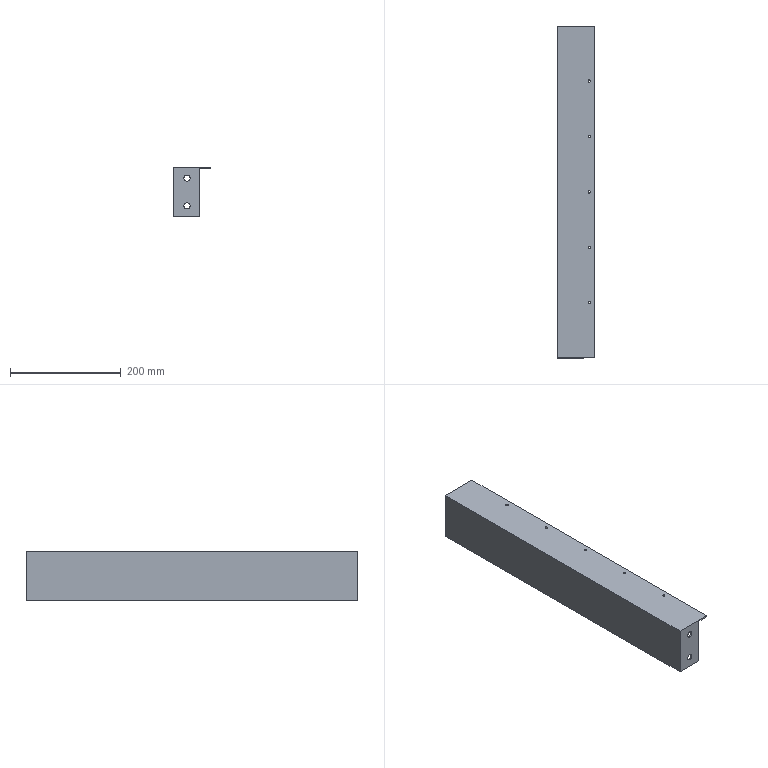Part | SolidWorks | features BaseBody 1 | 1 solid | 32 faces | box 68 x 599 x 90 mm | volume 277615 mm3 | cylinder 18 | plane 14 | commonest cylinder face diameters 4.4 x10 11 x8
STEP:
#1=CARTESIAN_POINT('',(202.746,-3340.973,1407.471));
#2=VERTEX_POINT('',#1);
#3=CARTESIAN_POINT('',(207.146,-3340.973,1407.471));
#4=VERTEX_POINT('',#3);
#5=CARTESIAN_POINT('',(204.946,-3340.973,1407.471));
#6=DIRECTION('',(0.,0.,1.));
#7=DIRECTION('',(1.,0.,0.));
#8=AXIS2_PLACEMENT_3D('',#5,#6,#7);
#9=CIRCLE('',#8,2.2);
#10=EDGE_CURVE('',#2,#4,#9,.T.);
#11=ORIENTED_EDGE('',*,*,#10,.F.);
#12=CARTESIAN_POINT('',(202.746,-3340.973,1409.971));
#13=VERTEX_POINT('',#12);
#14=CARTESIAN_POINT('',(202.746,-3340.973,1429.62));
#15=DIRECTION('',(0.,0.,1.));
#16=VECTOR('',#15,1000.);
#17=LINE('',#14,#16);
#18=EDGE_CURVE('',#2,#13,#17,.T.);
#19=ORIENTED_EDGE('',*,*,#18,.T.);
#20=CARTESIAN_POINT('',(207.146,-3340.973,1409.971));
#21=VERTEX_POINT('',#20);
#22=CARTESIAN_POINT('',(204.946,-3340.973,1409.971));
#23=DIRECTION('',(0.,0.,-1.));
#24=DIRECTION('',(1.,0.,0.));
#25=AXIS2_PLACEMENT_3D('',#22,#23,#24);
#26=CIRCLE('',#25,2.2);
#27=EDGE_CURVE('',#21,#13,#26,.T.);
#28=ORIENTED_EDGE('',*,*,#27,.F.);
#29=CARTESIAN_POINT('',(207.146,-3340.973,1429.62));
#30=DIRECTION('',(0.,0.,1.));
#31=VECTOR('',#30,1000.);
#32=LINE('',#29,#31);
#33=EDGE_CURVE('',#4,#21,#32,.T.);
#34=ORIENTED_EDGE('',*,*,#33,.F.);
#35=EDGE_LOOP('',(#11,#19,#28,#34));
#36=FACE_OUTER_BOUND('',#35,.T.);
#37=CARTESIAN_POINT('',(204.946,-3340.973,1429.62));
#38=DIRECTION('',(0.,0.,1.));
#39=DIRECTION('',(1.,0.,0.));
#40=AXIS2_PLACEMENT_3D('',#37,#38,#39);
#41=CYLINDRICAL_SURFACE('',#40,2.2);
#42=ADVANCED_FACE('',(#36),#41,.F.);
#43=CARTESIAN_POINT('',(202.746,-3140.973,1407.471));
#44=VERTEX_POINT('',#43);
#45=CARTESIAN_POINT('',(207.146,-3140.973,1407.471));
#46=VERTEX_POINT('',#45);
#47=CARTESIAN_POINT('',(204.946,-3140.973,1407.471));
#48=DIRECTION('',(0.,0.,1.));
#49=DIRECTION('',(1.,0.,0.));
#50=AXIS2_PLACEMENT_3D('',#47,#48,#49);
#51=CIRCLE('',#50,2.2);
#52=EDGE_CURVE('',#44,#46,#51,.T.);
#53=ORIENTED_EDGE('',*,*,#52,.F.);
#54=CARTESIAN_POINT('',(202.746,-3140.973,1409.971));
#55=VERTEX_POINT('',#54);
#56=CARTESIAN_POINT('',(202.746,-3140.973,1429.62));
#57=DIRECTION('',(0.,0.,1.));
#58=VECTOR('',#57,1000.);
#59=LINE('',#56,#58);
#60=EDGE_CURVE('',#44,#55,#59,.T.);
#61=ORIENTED_EDGE('',*,*,#60,.T.);
#62=CARTESIAN_POINT('',(207.146,-3140.973,1409.971));
#63=VERTEX_POINT('',#62);
#64=CARTESIAN_POINT('',(204.946,-3140.973,1409.971));
#65=DIRECTION('',(0.,0.,-1.));
#66=DIRECTION('',(1.,0.,0.));
#67=AXIS2_PLACEMENT_3D('',#64,#65,#66);
#68=CIRCLE('',#67,2.2);
#69=EDGE_CURVE('',#63,#55,#68,.T.);
#70=ORIENTED_EDGE('',*,*,#69,.F.);
#71=CARTESIAN_POINT('',(207.146,-3140.973,1429.62));
#72=DIRECTION('',(0.,0.,1.));
#73=VECTOR('',#72,1000.);
#74=LINE('',#71,#73);
#75=EDGE_CURVE('',#46,#63,#74,.T.);
#76=ORIENTED_EDGE('',*,*,#75,.F.);
#77=EDGE_LOOP('',(#53,#61,#70,#76));
#78=FACE_OUTER_BOUND('',#77,.T.);
#79=CARTESIAN_POINT('',(204.946,-3140.973,1429.62));
#80=DIRECTION('',(0.,0.,1.));
#81=DIRECTION('',(1.,0.,0.));
#82=AXIS2_PLACEMENT_3D('',#79,#80,#81);
#83=CYLINDRICAL_SURFACE('',#82,2.2);
#84=ADVANCED_FACE('',(#78),#83,.F.);
#85=CARTESIAN_POINT('',(202.746,-3540.973,1407.471));
#86=VERTEX_POINT('',#85);
#87=CARTESIAN_POINT('',(207.146,-3540.973,1407.471));
#88=VERTEX_POINT('',#87);
#89=CARTESIAN_POINT('',(204.946,-3540.973,1407.471));
#90=DIRECTION('',(0.,0.,1.));
#91=DIRECTION('',(1.,0.,0.));
#92=AXIS2_PLACEMENT_3D('',#89,#90,#91);
#93=CIRCLE('',#92,2.2);
#94=EDGE_CURVE('',#86,#88,#93,.T.);
#95=ORIENTED_EDGE('',*,*,#94,.F.);
#96=CARTESIAN_POINT('',(202.746,-3540.973,1409.971));
#97=VERTEX_POINT('',#96);
#98=CARTESIAN_POINT('',(202.746,-3540.973,1429.62));
#99=DIRECTION('',(0.,0.,1.));
#100=VECTOR('',#99,1000.);
#101=LINE('',#98,#100);
#102=EDGE_CURVE('',#86,#97,#101,.T.);
#103=ORIENTED_EDGE('',*,*,#102,.T.);
#104=CARTESIAN_POINT('',(207.146,-3540.973,1409.971));
#105=VERTEX_POINT('',#104);
#106=CARTESIAN_POINT('',(204.946,-3540.973,1409.971));
#107=DIRECTION('',(0.,0.,-1.));
#108=DIRECTION('',(1.,0.,0.));
#109=AXIS2_PLACEMENT_3D('',#106,#107,#108);
#110=CIRCLE('',#109,2.2);
#111=EDGE_CURVE('',#105,#97,#110,.T.);
#112=ORIENTED_EDGE('',*,*,#111,.F.);
#113=CARTESIAN_POINT('',(207.146,-3540.973,1429.62));
#114=DIRECTION('',(0.,0.,1.));
#115=VECTOR('',#114,1000.);
#116=LINE('',#113,#115);
#117=EDGE_CURVE('',#88,#105,#116,.T.);
#118=ORIENTED_EDGE('',*,*,#117,.F.);
#119=EDGE_LOOP('',(#95,#103,#112,#118));
#120=FACE_OUTER_BOUND('',#119,.T.);
#121=CARTESIAN_POINT('',(204.946,-3540.973,1429.62));
#122=DIRECTION('',(0.,0.,1.));
#123=DIRECTION('',(1.,0.,0.));
#124=AXIS2_PLACEMENT_3D('',#121,#122,#123);
#125=CYLINDRICAL_SURFACE('',#124,2.2);
#126=ADVANCED_FACE('',(#120),#125,.F.);
#127=CARTESIAN_POINT('',(202.746,-3440.973,1407.471));
#128=VERTEX_POINT('',#127);
#129=CARTESIAN_POINT('',(207.146,-3440.973,1407.471));
#130=VERTEX_POINT('',#129);
#131=CARTESIAN_POINT('',(204.946,-3440.973,1407.471));
#132=DIRECTION('',(0.,0.,1.));
#133=DIRECTION('',(1.,0.,0.));
#134=AXIS2_PLACEMENT_3D('',#131,#132,#133);
#135=CIRCLE('',#134,2.2);
#136=EDGE_CURVE('',#128,#130,#135,.T.);
#137=ORIENTED_EDGE('',*,*,#136,.F.);
#138=CARTESIAN_POINT('',(202.746,-3440.973,1409.971));
#139=VERTEX_POINT('',#138);
#140=CARTESIAN_POINT('',(202.746,-3440.973,1429.62));
#141=DIRECTION('',(0.,0.,1.));
#142=VECTOR('',#141,1000.);
#143=LINE('',#140,#142);
#144=EDGE_CURVE('',#128,#139,#143,.T.);
#145=ORIENTED_EDGE('',*,*,#144,.T.);
#146=CARTESIAN_POINT('',(207.146,-3440.973,1409.971));
#147=VERTEX_POINT('',#146);
#148=CARTESIAN_POINT('',(204.946,-3440.973,1409.971));
#149=DIRECTION('',(0.,0.,-1.));
#150=DIRECTION('',(1.,0.,0.));
#151=AXIS2_PLACEMENT_3D('',#148,#149,#150);
#152=CIRCLE('',#151,2.2);
#153=EDGE_CURVE('',#147,#139,#152,.T.);
#154=ORIENTED_EDGE('',*,*,#153,.F.);
#155=CARTESIAN_POINT('',(207.146,-3440.973,1429.62));
#156=DIRECTION('',(0.,0.,1.));
#157=VECTOR('',#156,1000.);
#158=LINE('',#155,#157);
#159=EDGE_CURVE('',#130,#147,#158,.T.);
#160=ORIENTED_EDGE('',*,*,#159,.F.);
#161=EDGE_LOOP('',(#137,#145,#154,#160));
#162=FACE_OUTER_BOUND('',#161,.T.);
#163=CARTESIAN_POINT('',(204.946,-3440.973,1429.62));
#164=DIRECTION('',(0.,0.,1.));
#165=DIRECTION('',(1.,0.,0.));
#166=AXIS2_PLACEMENT_3D('',#163,#164,#165);
#167=CYLINDRICAL_SURFACE('',#166,2.2);
#168=ADVANCED_FACE('',(#162),#167,.F.);
#169=CARTESIAN_POINT('',(202.746,-3240.973,1407.471));
#170=VERTEX_POINT('',#169);
#171=CARTESIAN_POINT('',(207.146,-3240.973,1407.471));
#172=VERTEX_POINT('',#171);
#173=CARTESIAN_POINT('',(204.946,-3240.973,1407.471));
#174=DIRECTION('',(0.,0.,1.));
#175=DIRECTION('',(1.,0.,0.));
#176=AXIS2_PLACEMENT_3D('',#173,#174,#175);
#177=CIRCLE('',#176,2.2);
#178=EDGE_CURVE('',#170,#172,#177,.T.);
#179=ORIENTED_EDGE('',*,*,#178,.F.);
#180=CARTESIAN_POINT('',(202.746,-3240.973,1409.971));
#181=VERTEX_POINT('',#180);
#182=CARTESIAN_POINT('',(202.746,-3240.973,1429.62));
#183=DIRECTION('',(0.,0.,1.));
#184=VECTOR('',#183,1000.);
#185=LINE('',#182,#184);
#186=EDGE_CURVE('',#170,#181,#185,.T.);
#187=ORIENTED_EDGE('',*,*,#186,.T.);
#188=CARTESIAN_POINT('',(207.146,-3240.973,1409.971));
#189=VERTEX_POINT('',#188);
#190=CARTESIAN_POINT('',(204.946,-3240.973,1409.971));
#191=DIRECTION('',(0.,0.,-1.));
#192=DIRECTION('',(1.,0.,0.));
#193=AXIS2_PLACEMENT_3D('',#190,#191,#192);
#194=CIRCLE('',#193,2.2);
#195=EDGE_CURVE('',#189,#181,#194,.T.);
#196=ORIENTED_EDGE('',*,*,#195,.F.);
#197=CARTESIAN_POINT('',(207.146,-3240.973,1429.62));
#198=DIRECTION('',(0.,0.,1.));
#199=VECTOR('',#198,1000.);
#200=LINE('',#197,#199);
#201=EDGE_CURVE('',#172,#189,#200,.T.);
#202=ORIENTED_EDGE('',*,*,#201,.F.);
#203=EDGE_LOOP('',(#179,#187,#196,#202));
#204=FACE_OUTER_BOUND('',#203,.T.);
#205=CARTESIAN_POINT('',(204.946,-3240.973,1429.62));
#206=DIRECTION('',(0.,0.,1.));
#207=DIRECTION('',(1.,0.,0.));
#208=AXIS2_PLACEMENT_3D('',#205,#206,#207);
#209=CYLINDRICAL_SURFACE('',#208,2.2);
#210=ADVANCED_FACE('',(#204),#209,.F.);
#211=CARTESIAN_POINT('',(171.946,-3640.473,1395.471));
#212=VERTEX_POINT('',#211);
#213=CARTESIAN_POINT('',(171.946,-3640.473,1384.471));
#214=VERTEX_POINT('',#213);
#215=CARTESIAN_POINT('',(171.946,-3640.473,1389.971));
#216=DIRECTION('',(0.,-1.,0.));
#217=DIRECTION('',(0.,0.,1.));
#218=AXIS2_PLACEMENT_3D('',#215,#216,#217);
#219=CIRCLE('',#218,5.5);
#220=EDGE_CURVE('',#212,#214,#219,.T.);
#221=ORIENTED_EDGE('',*,*,#220,.T.);
#222=CARTESIAN_POINT('',(171.946,-3637.973,1384.471));
#223=VERTEX_POINT('',#222);
#224=CARTESIAN_POINT('',(171.946,-3640.473,1384.471));
#225=DIRECTION('',(0.,1.,0.));
#226=VECTOR('',#225,1000.);
#227=LINE('',#224,#226);
#228=EDGE_CURVE('',#214,#223,#227,.T.);
#229=ORIENTED_EDGE('',*,*,#228,.T.);
#230=CARTESIAN_POINT('',(171.946,-3637.973,1395.471));
#231=VERTEX_POINT('',#230);
#232=CARTESIAN_POINT('',(171.946,-3637.973,1389.971));
#233=DIRECTION('',(0.,1.,0.));
#234=DIRECTION('',(0.,0.,1.));
#235=AXIS2_PLACEMENT_3D('',#232,#233,#234);
#236=CIRCLE('',#235,5.5);
#237=EDGE_CURVE('',#223,#231,#236,.T.);
#238=ORIENTED_EDGE('',*,*,#237,.T.);
#239=CARTESIAN_POINT('',(171.946,-3640.473,1395.471));
#240=DIRECTION('',(0.,1.,0.));
#241=VECTOR('',#240,1000.);
#242=LINE('',#239,#241);
#243=EDGE_CURVE('',#212,#231,#242,.T.);
#244=ORIENTED_EDGE('',*,*,#243,.F.);
#245=EDGE_LOOP('',(#221,#229,#238,#244));
#246=FACE_OUTER_BOUND('',#245,.T.);
#247=CARTESIAN_POINT('',(171.946,-3640.473,1389.971));
#248=DIRECTION('',(0.,1.,0.));
#249=DIRECTION('',(0.,0.,1.));
#250=AXIS2_PLACEMENT_3D('',#247,#248,#249);
#251=CYLINDRICAL_SURFACE('',#250,5.5);
#252=ADVANCED_FACE('',(#246),#251,.F.);
#253=CARTESIAN_POINT('',(171.946,-3640.473,1345.471));
#254=VERTEX_POINT('',#253);
#255=CARTESIAN_POINT('',(171.946,-3640.473,1334.471));
#256=VERTEX_POINT('',#255);
#257=CARTESIAN_POINT('',(171.946,-3640.473,1339.971));
#258=DIRECTION('',(0.,-1.,0.));
#259=DIRECTION('',(0.,0.,1.));
#260=AXIS2_PLACEMENT_3D('',#257,#258,#259);
#261=CIRCLE('',#260,5.5);
#262=EDGE_CURVE('',#254,#256,#261,.T.);
#263=ORIENTED_EDGE('',*,*,#262,.T.);
#264=CARTESIAN_POINT('',(171.946,-3637.973,1334.471));
#265=VERTEX_POINT('',#264);
#266=CARTESIAN_POINT('',(171.946,-3640.473,1334.471));
#267=DIRECTION('',(0.,1.,0.));
#268=VECTOR('',#267,1000.);
#269=LINE('',#266,#268);
#270=EDGE_CURVE('',#256,#265,#269,.T.);
#271=ORIENTED_EDGE('',*,*,#270,.T.);
#272=CARTESIAN_POINT('',(171.946,-3637.973,1345.471));
#273=VERTEX_POINT('',#272);
#274=CARTESIAN_POINT('',(171.946,-3637.973,1339.971));
#275=DIRECTION('',(0.,1.,0.));
#276=DIRECTION('',(0.,0.,1.));
#277=AXIS2_PLACEMENT_3D('',#274,#275,#276);
#278=CIRCLE('',#277,5.5);
#279=EDGE_CURVE('',#265,#273,#278,.T.);
#280=ORIENTED_EDGE('',*,*,#279,.T.);
#281=CARTESIAN_POINT('',(171.946,-3640.473,1345.471));
#282=DIRECTION('',(0.,1.,0.));
#283=VECTOR('',#282,1000.);
#284=LINE('',#281,#283);
#285=EDGE_CURVE('',#254,#273,#284,.T.);
#286=ORIENTED_EDGE('',*,*,#285,.F.);
#287=EDGE_LOOP('',(#263,#271,#280,#286));
#288=FACE_OUTER_BOUND('',#287,.T.);
#289=CARTESIAN_POINT('',(171.946,-3640.473,1339.971));
#290=DIRECTION('',(0.,1.,0.));
#291=DIRECTION('',(0.,0.,1.));
#292=AXIS2_PLACEMENT_3D('',#289,#290,#291);
#293=CYLINDRICAL_SURFACE('',#292,5.5);
#294=ADVANCED_FACE('',(#288),#293,.F.);
#295=CARTESIAN_POINT('',(171.946,-3043.973,1384.471));
#296=VERTEX_POINT('',#295);
#297=CARTESIAN_POINT('',(171.946,-3043.973,1395.471));
#298=VERTEX_POINT('',#297);
#299=CARTESIAN_POINT('',(171.946,-3043.973,1389.971));
#300=DIRECTION('',(0.,1.,0.));
#301=DIRECTION('',(0.,0.,1.));
#302=AXIS2_PLACEMENT_3D('',#299,#300,#301);
#303=CIRCLE('',#302,5.5);
#304=EDGE_CURVE('',#296,#298,#303,.T.);
#305=ORIENTED_EDGE('',*,*,#304,.F.);
#306=CARTESIAN_POINT('',(171.946,-3041.473,1384.471));
#307=VERTEX_POINT('',#306);
#308=CARTESIAN_POINT('',(171.946,-3043.973,1384.471));
#309=DIRECTION('',(0.,1.,0.));
#310=VECTOR('',#309,1000.);
#311=LINE('',#308,#310);
#312=EDGE_CURVE('',#296,#307,#311,.T.);
#313=ORIENTED_EDGE('',*,*,#312,.T.);
#314=CARTESIAN_POINT('',(171.946,-3041.473,1395.471));
#315=VERTEX_POINT('',#314);
#316=CARTESIAN_POINT('',(171.946,-3041.473,1389.971));
#317=DIRECTION('',(0.,1.,0.));
#318=DIRECTION('',(0.,0.,1.));
#319=AXIS2_PLACEMENT_3D('',#316,#317,#318);
#320=CIRCLE('',#319,5.5);
#321=EDGE_CURVE('',#307,#315,#320,.T.);
#322=ORIENTED_EDGE('',*,*,#321,.T.);
#323=CARTESIAN_POINT('',(171.946,-3043.973,1395.471));
#324=DIRECTION('',(0.,1.,0.));
#325=VECTOR('',#324,1000.);
#326=LINE('',#323,#325);
#327=EDGE_CURVE('',#298,#315,#326,.T.);
#328=ORIENTED_EDGE('',*,*,#327,.F.);
#329=EDGE_LOOP('',(#305,#313,#322,#328));
#330=FACE_OUTER_BOUND('',#329,.T.);
#331=CARTESIAN_POINT('',(171.946,-3043.973,1389.971));
#332=DIRECTION('',(0.,1.,0.));
#333=DIRECTION('',(0.,0.,1.));
#334=AXIS2_PLACEMENT_3D('',#331,#332,#333);
#335=CYLINDRICAL_SURFACE('',#334,5.5);
#336=ADVANCED_FACE('',(#330),#335,.F.);
#337=CARTESIAN_POINT('',(171.946,-3043.973,1334.471));
#338=VERTEX_POINT('',#337);
#339=CARTESIAN_POINT('',(171.946,-3043.973,1345.471));
#340=VERTEX_POINT('',#339);
#341=CARTESIAN_POINT('',(171.946,-3043.973,1339.971));
#342=DIRECTION('',(0.,1.,0.));
#343=DIRECTION('',(0.,0.,1.));
#344=AXIS2_PLACEMENT_3D('',#341,#342,#343);
#345=CIRCLE('',#344,5.5);
#346=EDGE_CURVE('',#338,#340,#345,.T.);
#347=ORIENTED_EDGE('',*,*,#346,.F.);
#348=CARTESIAN_POINT('',(171.946,-3041.473,1334.471));
#349=VERTEX_POINT('',#348);
#350=CARTESIAN_POINT('',(171.946,-3043.973,1334.471));
#351=DIRECTION('',(0.,1.,0.));
#352=VECTOR('',#351,1000.);
#353=LINE('',#350,#352);
#354=EDGE_CURVE('',#338,#349,#353,.T.);
#355=ORIENTED_EDGE('',*,*,#354,.T.);
#356=CARTESIAN_POINT('',(171.946,-3041.473,1345.471));
#357=VERTEX_POINT('',#356);
#358=CARTESIAN_POINT('',(171.946,-3041.473,1339.971));
#359=DIRECTION('',(0.,1.,0.));
#360=DIRECTION('',(0.,0.,1.));
#361=AXIS2_PLACEMENT_3D('',#358,#359,#360);
#362=CIRCLE('',#361,5.5);
#363=EDGE_CURVE('',#349,#357,#362,.T.);
#364=ORIENTED_EDGE('',*,*,#363,.T.);
#365=CARTESIAN_POINT('',(171.946,-3043.973,1345.471));
#366=DIRECTION('',(0.,1.,0.));
#367=VECTOR('',#366,1000.);
#368=LINE('',#365,#367);
#369=EDGE_CURVE('',#340,#357,#368,.T.);
#370=ORIENTED_EDGE('',*,*,#369,.F.);
#371=EDGE_LOOP('',(#347,#355,#364,#370));
#372=FACE_OUTER_BOUND('',#371,.T.);
#373=CARTESIAN_POINT('',(171.946,-3043.973,1339.971));
#374=DIRECTION('',(0.,1.,0.));
#375=DIRECTION('',(0.,0.,1.));
#376=AXIS2_PLACEMENT_3D('',#373,#374,#375);
#377=CYLINDRICAL_SURFACE('',#376,5.5);
#378=ADVANCED_FACE('',(#372),#377,.F.);
#379=CARTESIAN_POINT('',(146.946,-3640.473,1319.971));
#380=VERTEX_POINT('',#379);
#381=CARTESIAN_POINT('',(146.946,-3640.473,1409.971));
#382=VERTEX_POINT('',#381);
#383=CARTESIAN_POINT('',(146.946,-3640.473,1409.971));
#384=DIRECTION('',(0.,0.,1.));
#385=VECTOR('',#384,1000.);
#386=LINE('',#383,#385);
#387=EDGE_CURVE('',#380,#382,#386,.T.);
#388=ORIENTED_EDGE('',*,*,#387,.T.);
#389=CARTESIAN_POINT('',(146.946,-3041.473,1409.971));
#390=VERTEX_POINT('',#389);
#391=CARTESIAN_POINT('',(146.946,-3043.973,1409.971));
#392=DIRECTION('',(0.,1.,0.));
#393=VECTOR('',#392,1000.);
#394=LINE('',#391,#393);
#395=EDGE_CURVE('',#382,#390,#394,.T.);
#396=ORIENTED_EDGE('',*,*,#395,.T.);
#397=CARTESIAN_POINT('',(146.946,-3041.473,1319.971));
#398=VERTEX_POINT('',#397);
#399=CARTESIAN_POINT('',(146.946,-3041.473,1409.971));
#400=DIRECTION('',(0.,0.,-1.));
#401=VECTOR('',#400,1000.);
#402=LINE('',#399,#401);
#403=EDGE_CURVE('',#390,#398,#402,.T.);
#404=ORIENTED_EDGE('',*,*,#403,.T.);
#405=CARTESIAN_POINT('',(146.946,-3043.973,1319.971));
#406=DIRECTION('',(0.,-1.,0.));
#407=VECTOR('',#406,1000.);
#408=LINE('',#405,#407);
#409=EDGE_CURVE('',#398,#380,#408,.T.);
#410=ORIENTED_EDGE('',*,*,#409,.T.);
#411=EDGE_LOOP('',(#388,#396,#404,#410));
#412=FACE_OUTER_BOUND('',#411,.T.);
#413=CARTESIAN_POINT('',(146.946,-3043.973,1409.971));
#414=DIRECTION('',(-1.,0.,0.));
#415=DIRECTION('',(0.,0.,1.));
#416=AXIS2_PLACEMENT_3D('',#413,#414,#415);
#417=PLANE('',#416);
#418=ADVANCED_FACE('',(#412),#417,.T.);
#419=CARTESIAN_POINT('',(214.946,-3640.473,1409.971));
#420=VERTEX_POINT('',#419);
#421=CARTESIAN_POINT('',(194.946,-3640.473,1409.971));
#422=DIRECTION('',(1.,0.,0.));
#423=VECTOR('',#422,1000.);
#424=LINE('',#421,#423);
#425=EDGE_CURVE('',#382,#420,#424,.T.);
#426=ORIENTED_EDGE('',*,*,#425,.T.);
#427=CARTESIAN_POINT('',(214.946,-3041.473,1409.971));
#428=VERTEX_POINT('',#427);
#429=CARTESIAN_POINT('',(214.946,-3043.973,1409.971));
#430=DIRECTION('',(0.,1.,0.));
#431=VECTOR('',#430,1000.);
#432=LINE('',#429,#431);
#433=EDGE_CURVE('',#420,#428,#432,.T.);
#434=ORIENTED_EDGE('',*,*,#433,.T.);
#435=CARTESIAN_POINT('',(194.946,-3041.473,1409.971));
#436=DIRECTION('',(-1.,0.,0.));
#437=VECTOR('',#436,1000.);
#438=LINE('',#435,#437);
#439=EDGE_CURVE('',#428,#390,#438,.T.);
#440=ORIENTED_EDGE('',*,*,#439,.T.);
#441=ORIENTED_EDGE('',*,*,#395,.F.);
#442=EDGE_LOOP('',(#426,#434,#440,#441));
#443=FACE_OUTER_BOUND('',#442,.T.);
#444=ORIENTED_EDGE('',*,*,#27,.T.);
#445=CARTESIAN_POINT('',(204.946,-3340.973,1409.971));
#446=DIRECTION('',(0.,0.,-1.));
#447=DIRECTION('',(1.,0.,0.));
#448=AXIS2_PLACEMENT_3D('',#445,#446,#447);
#449=CIRCLE('',#448,2.2);
#450=EDGE_CURVE('',#13,#21,#449,.T.);
#451=ORIENTED_EDGE('',*,*,#450,.T.);
#452=EDGE_LOOP('',(#444,#451));
#453=FACE_BOUND('',#452,.T.);
#454=ORIENTED_EDGE('',*,*,#69,.T.);
#455=CARTESIAN_POINT('',(204.946,-3140.973,1409.971));
#456=DIRECTION('',(0.,0.,-1.));
#457=DIRECTION('',(1.,0.,0.));
#458=AXIS2_PLACEMENT_3D('',#455,#456,#457);
#459=CIRCLE('',#458,2.2);
#460=EDGE_CURVE('',#55,#63,#459,.T.);
#461=ORIENTED_EDGE('',*,*,#460,.T.);
#462=EDGE_LOOP('',(#454,#461));
#463=FACE_BOUND('',#462,.T.);
#464=ORIENTED_EDGE('',*,*,#111,.T.);
#465=CARTESIAN_POINT('',(204.946,-3540.973,1409.971));
#466=DIRECTION('',(0.,0.,-1.));
#467=DIRECTION('',(1.,0.,0.));
#468=AXIS2_PLACEMENT_3D('',#465,#466,#467);
#469=CIRCLE('',#468,2.2);
#470=EDGE_CURVE('',#97,#105,#469,.T.);
#471=ORIENTED_EDGE('',*,*,#470,.T.);
#472=EDGE_LOOP('',(#464,#471));
#473=FACE_BOUND('',#472,.T.);
#474=ORIENTED_EDGE('',*,*,#153,.T.);
#475=CARTESIAN_POINT('',(204.946,-3440.973,1409.971));
#476=DIRECTION('',(0.,0.,-1.));
#477=DIRECTION('',(1.,0.,0.));
#478=AXIS2_PLACEMENT_3D('',#475,#476,#477);
#479=CIRCLE('',#478,2.2);
#480=EDGE_CURVE('',#139,#147,#479,.T.);
#481=ORIENTED_EDGE('',*,*,#480,.T.);
#482=EDGE_LOOP('',(#474,#481));
#483=FACE_BOUND('',#482,.T.);
#484=ORIENTED_EDGE('',*,*,#195,.T.);
#485=CARTESIAN_POINT('',(204.946,-3240.973,1409.971));
#486=DIRECTION('',(0.,0.,-1.));
#487=DIRECTION('',(1.,0.,0.));
#488=AXIS2_PLACEMENT_3D('',#485,#486,#487);
#489=CIRCLE('',#488,2.2);
#490=EDGE_CURVE('',#181,#189,#489,.T.);
#491=ORIENTED_EDGE('',*,*,#490,.T.);
#492=EDGE_LOOP('',(#484,#491));
#493=FACE_BOUND('',#492,.T.);
#494=CARTESIAN_POINT('',(194.946,-3043.973,1409.971));
#495=DIRECTION('',(0.,0.,1.));
#496=DIRECTION('',(1.,0.,0.));
#497=AXIS2_PLACEMENT_3D('',#494,#495,#496);
#498=PLANE('',#497);
#499=ADVANCED_FACE('',(#443,#453,#463,#473,#483,#493),#498,.T.);
#500=ORIENTED_EDGE('',*,*,#220,.F.);
#501=CARTESIAN_POINT('',(171.946,-3640.473,1389.971));
#502=DIRECTION('',(0.,-1.,0.));
#503=DIRECTION('',(0.,0.,1.));
#504=AXIS2_PLACEMENT_3D('',#501,#502,#503);
#505=CIRCLE('',#504,5.5);
#506=EDGE_CURVE('',#214,#212,#505,.T.);
#507=ORIENTED_EDGE('',*,*,#506,.F.);
#508=EDGE_LOOP('',(#500,#507));
#509=FACE_BOUND('',#508,.T.);
#510=ORIENTED_EDGE('',*,*,#262,.F.);
#511=CARTESIAN_POINT('',(171.946,-3640.473,1339.971));
#512=DIRECTION('',(0.,-1.,0.));
#513=DIRECTION('',(0.,0.,1.));
#514=AXIS2_PLACEMENT_3D('',#511,#512,#513);
#515=CIRCLE('',#514,5.5);
#516=EDGE_CURVE('',#256,#254,#515,.T.);
#517=ORIENTED_EDGE('',*,*,#516,.F.);
#518=EDGE_LOOP('',(#510,#517));
#519=FACE_BOUND('',#518,.T.);
#520=CARTESIAN_POINT('',(214.946,-3640.473,1407.471));
#521=VERTEX_POINT('',#520);
#522=CARTESIAN_POINT('',(214.946,-3640.473,1364.971));
#523=DIRECTION('',(0.,0.,-1.));
#524=VECTOR('',#523,1000.);
#525=LINE('',#522,#524);
#526=EDGE_CURVE('',#420,#521,#525,.T.);
#527=ORIENTED_EDGE('',*,*,#526,.F.);
#528=ORIENTED_EDGE('',*,*,#425,.F.);
#529=ORIENTED_EDGE('',*,*,#387,.F.);
#530=CARTESIAN_POINT('',(194.946,-3640.473,1319.971));
#531=VERTEX_POINT('',#530);
#532=CARTESIAN_POINT('',(170.946,-3640.473,1319.971));
#533=DIRECTION('',(-1.,0.,0.));
#534=VECTOR('',#533,1000.);
#535=LINE('',#532,#534);
#536=EDGE_CURVE('',#531,#380,#535,.T.);
#537=ORIENTED_EDGE('',*,*,#536,.F.);
#538=CARTESIAN_POINT('',(194.946,-3640.473,1407.471));
#539=VERTEX_POINT('',#538);
#540=CARTESIAN_POINT('',(194.946,-3640.473,1364.971));
#541=DIRECTION('',(0.,0.,-1.));
#542=VECTOR('',#541,1000.);
#543=LINE('',#540,#542);
#544=EDGE_CURVE('',#539,#531,#543,.T.);
#545=ORIENTED_EDGE('',*,*,#544,.F.);
#546=CARTESIAN_POINT('',(170.946,-3640.473,1407.471));
#547=DIRECTION('',(-1.,0.,0.));
#548=VECTOR('',#547,1000.);
#549=LINE('',#546,#548);
#550=EDGE_CURVE('',#521,#539,#549,.T.);
#551=ORIENTED_EDGE('',*,*,#550,.F.);
#552=EDGE_LOOP('',(#527,#528,#529,#537,#545,#551));
#553=FACE_OUTER_BOUND('',#552,.T.);
#554=CARTESIAN_POINT('',(170.946,-3640.473,1364.971));
#555=DIRECTION('',(0.,1.,0.));
#556=DIRECTION('',(0.,0.,1.));
#557=AXIS2_PLACEMENT_3D('',#554,#555,#556);
#558=PLANE('',#557);
#559=ADVANCED_FACE('',(#509,#519,#553),#558,.F.);
#560=CARTESIAN_POINT('',(194.946,-3043.973,1319.971));
#561=VERTEX_POINT('',#560);
#562=CARTESIAN_POINT('',(166.946,-3043.973,1319.971));
#563=VERTEX_POINT('',#562);
#564=CARTESIAN_POINT('',(146.946,-3043.973,1319.971));
#565=DIRECTION('',(-1.,0.,0.));
#566=VECTOR('',#565,1000.);
#567=LINE('',#564,#566);
#568=EDGE_CURVE('',#561,#563,#567,.T.);
#569=ORIENTED_EDGE('',*,*,#568,.T.);
#570=CARTESIAN_POINT('',(166.946,-3637.973,1319.971));
#571=VERTEX_POINT('',#570);
#572=CARTESIAN_POINT('',(166.946,-3043.973,1319.971));
#573=DIRECTION('',(0.,-1.,0.));
#574=VECTOR('',#573,1000.);
#575=LINE('',#572,#574);
#576=EDGE_CURVE('',#563,#571,#575,.T.);
#577=ORIENTED_EDGE('',*,*,#576,.T.);
#578=CARTESIAN_POINT('',(194.946,-3637.973,1319.971));
#579=VERTEX_POINT('',#578);
#580=CARTESIAN_POINT('',(146.946,-3637.973,1319.971));
#581=DIRECTION('',(1.,0.,0.));
#582=VECTOR('',#581,1000.);
#583=LINE('',#580,#582);
#584=EDGE_CURVE('',#571,#579,#583,.T.);
#585=ORIENTED_EDGE('',*,*,#584,.T.);
#586=CARTESIAN_POINT('',(194.946,-3043.973,1319.971));
#587=DIRECTION('',(0.,-1.,0.));
#588=VECTOR('',#587,1000.);
#589=LINE('',#586,#588);
#590=EDGE_CURVE('',#579,#531,#589,.T.);
#591=ORIENTED_EDGE('',*,*,#590,.T.);
#592=ORIENTED_EDGE('',*,*,#536,.T.);
#593=ORIENTED_EDGE('',*,*,#409,.F.);
#594=CARTESIAN_POINT('',(194.946,-3041.473,1319.971));
#595=VERTEX_POINT('',#594);
#596=CARTESIAN_POINT('',(146.946,-3041.473,1319.971));
#597=DIRECTION('',(1.,0.,0.));
#598=VECTOR('',#597,1000.);
#599=LINE('',#596,#598);
#600=EDGE_CURVE('',#398,#595,#599,.T.);
#601=ORIENTED_EDGE('',*,*,#600,.T.);
#602=CARTESIAN_POINT('',(194.946,-3043.973,1319.971));
#603=DIRECTION('',(0.,-1.,0.));
#604=VECTOR('',#603,1000.);
#605=LINE('',#602,#604);
#606=EDGE_CURVE('',#595,#561,#605,.T.);
#607=ORIENTED_EDGE('',*,*,#606,.T.);
#608=EDGE_LOOP('',(#569,#577,#585,#591,#592,#593,#601,#607));
#609=FACE_OUTER_BOUND('',#608,.T.);
#610=CARTESIAN_POINT('',(146.946,-3043.973,1319.971));
#611=DIRECTION('',(0.,0.,-1.));
#612=DIRECTION('',(-1.,0.,0.));
#613=AXIS2_PLACEMENT_3D('',#610,#611,#612);
#614=PLANE('',#613);
#615=ADVANCED_FACE('',(#609),#614,.T.);
#616=CARTESIAN_POINT('',(194.946,-3041.473,1407.471));
#617=VERTEX_POINT('',#616);
#618=CARTESIAN_POINT('',(194.946,-3041.473,1364.971));
#619=DIRECTION('',(0.,0.,1.));
#620=VECTOR('',#619,1000.);
#621=LINE('',#618,#620);
#622=EDGE_CURVE('',#595,#617,#621,.T.);
#623=ORIENTED_EDGE('',*,*,#622,.F.);
#624=ORIENTED_EDGE('',*,*,#600,.F.);
#625=ORIENTED_EDGE('',*,*,#403,.F.);
#626=ORIENTED_EDGE('',*,*,#439,.F.);
#627=CARTESIAN_POINT('',(214.946,-3041.473,1407.471));
#628=VERTEX_POINT('',#627);
#629=CARTESIAN_POINT('',(214.946,-3041.473,1364.971));
#630=DIRECTION('',(0.,0.,1.));
#631=VECTOR('',#630,1000.);
#632=LINE('',#629,#631);
#633=EDGE_CURVE('',#628,#428,#632,.T.);
#634=ORIENTED_EDGE('',*,*,#633,.F.);
#635=CARTESIAN_POINT('',(170.946,-3041.473,1407.471));
#636=DIRECTION('',(1.,0.,0.));
#637=VECTOR('',#636,1000.);
#638=LINE('',#635,#637);
#639=EDGE_CURVE('',#617,#628,#638,.T.);
#640=ORIENTED_EDGE('',*,*,#639,.F.);
#641=EDGE_LOOP('',(#623,#624,#625,#626,#634,#640));
#642=FACE_OUTER_BOUND('',#641,.T.);
#643=CARTESIAN_POINT('',(171.946,-3041.473,1389.971));
#644=DIRECTION('',(0.,1.,0.));
#645=DIRECTION('',(0.,0.,1.));
#646=AXIS2_PLACEMENT_3D('',#643,#644,#645);
#647=CIRCLE('',#646,5.5);
#648=EDGE_CURVE('',#315,#307,#647,.T.);
#649=ORIENTED_EDGE('',*,*,#648,.F.);
#650=ORIENTED_EDGE('',*,*,#321,.F.);
#651=EDGE_LOOP('',(#649,#650));
#652=FACE_BOUND('',#651,.T.);
#653=CARTESIAN_POINT('',(171.946,-3041.473,1339.971));
#654=DIRECTION('',(0.,1.,0.));
#655=DIRECTION('',(0.,0.,1.));
#656=AXIS2_PLACEMENT_3D('',#653,#654,#655);
#657=CIRCLE('',#656,5.5);
#658=EDGE_CURVE('',#357,#349,#657,.T.);
#659=ORIENTED_EDGE('',*,*,#658,.F.);
#660=ORIENTED_EDGE('',*,*,#363,.F.);
#661=EDGE_LOOP('',(#659,#660));
#662=FACE_BOUND('',#661,.T.);
#663=CARTESIAN_POINT('',(170.946,-3041.473,1364.971));
#664=DIRECTION('',(0.,-1.,0.));
#665=DIRECTION('',(1.,0.,0.));
#666=AXIS2_PLACEMENT_3D('',#663,#664,#665);
#667=PLANE('',#666);
#668=ADVANCED_FACE('',(#642,#652,#662),#667,.F.);
#669=ORIENTED_EDGE('',*,*,#433,.F.);
#670=ORIENTED_EDGE('',*,*,#526,.T.);
#671=CARTESIAN_POINT('',(214.946,-3043.973,1407.471));
#672=DIRECTION('',(0.,1.,0.));
#673=VECTOR('',#672,1000.);
#674=LINE('',#671,#673);
#675=EDGE_CURVE('',#521,#628,#674,.T.);
#676=ORIENTED_EDGE('',*,*,#675,.T.);
#677=ORIENTED_EDGE('',*,*,#633,.T.);
#678=EDGE_LOOP('',(#669,#670,#676,#677));
#679=FACE_OUTER_BOUND('',#678,.T.);
#680=CARTESIAN_POINT('',(214.946,-3043.973,1319.971));
#681=DIRECTION('',(1.,0.,0.));
#682=DIRECTION('',(0.,0.,-1.));
#683=AXIS2_PLACEMENT_3D('',#680,#681,#682);
#684=PLANE('',#683);
#685=ADVANCED_FACE('',(#679),#684,.T.);
#686=ORIENTED_EDGE('',*,*,#18,.F.);
#687=CARTESIAN_POINT('',(204.946,-3340.973,1407.471));
#688=DIRECTION('',(0.,0.,1.));
#689=DIRECTION('',(1.,0.,0.));
#690=AXIS2_PLACEMENT_3D('',#687,#688,#689);
#691=CIRCLE('',#690,2.2);
#692=EDGE_CURVE('',#4,#2,#691,.T.);
#693=ORIENTED_EDGE('',*,*,#692,.F.);
#694=ORIENTED_EDGE('',*,*,#33,.T.);
#695=ORIENTED_EDGE('',*,*,#450,.F.);
#696=EDGE_LOOP('',(#686,#693,#694,#695));
#697=FACE_OUTER_BOUND('',#696,.T.);
#698=CARTESIAN_POINT('',(204.946,-3340.973,1429.62));
#699=DIRECTION('',(0.,0.,1.));
#700=DIRECTION('',(1.,0.,0.));
#701=AXIS2_PLACEMENT_3D('',#698,#699,#700);
#702=CYLINDRICAL_SURFACE('',#701,2.2);
#703=ADVANCED_FACE('',(#697),#702,.F.);
#704=ORIENTED_EDGE('',*,*,#60,.F.);
#705=CARTESIAN_POINT('',(204.946,-3140.973,1407.471));
#706=DIRECTION('',(0.,0.,1.));
#707=DIRECTION('',(1.,0.,0.));
#708=AXIS2_PLACEMENT_3D('',#705,#706,#707);
#709=CIRCLE('',#708,2.2);
#710=EDGE_CURVE('',#46,#44,#709,.T.);
#711=ORIENTED_EDGE('',*,*,#710,.F.);
#712=ORIENTED_EDGE('',*,*,#75,.T.);
#713=ORIENTED_EDGE('',*,*,#460,.F.);
#714=EDGE_LOOP('',(#704,#711,#712,#713));
#715=FACE_OUTER_BOUND('',#714,.T.);
#716=CARTESIAN_POINT('',(204.946,-3140.973,1429.62));
#717=DIRECTION('',(0.,0.,1.));
#718=DIRECTION('',(1.,0.,0.));
#719=AXIS2_PLACEMENT_3D('',#716,#717,#718);
#720=CYLINDRICAL_SURFACE('',#719,2.2);
#721=ADVANCED_FACE('',(#715),#720,.F.);
#722=ORIENTED_EDGE('',*,*,#102,.F.);
#723=CARTESIAN_POINT('',(204.946,-3540.973,1407.471));
#724=DIRECTION('',(0.,0.,1.));
#725=DIRECTION('',(1.,0.,0.));
#726=AXIS2_PLACEMENT_3D('',#723,#724,#725);
#727=CIRCLE('',#726,2.2);
#728=EDGE_CURVE('',#88,#86,#727,.T.);
#729=ORIENTED_EDGE('',*,*,#728,.F.);
#730=ORIENTED_EDGE('',*,*,#117,.T.);
#731=ORIENTED_EDGE('',*,*,#470,.F.);
#732=EDGE_LOOP('',(#722,#729,#730,#731));
#733=FACE_OUTER_BOUND('',#732,.T.);
#734=CARTESIAN_POINT('',(204.946,-3540.973,1429.62));
#735=DIRECTION('',(0.,0.,1.));
#736=DIRECTION('',(1.,0.,0.));
#737=AXIS2_PLACEMENT_3D('',#734,#735,#736);
#738=CYLINDRICAL_SURFACE('',#737,2.2);
#739=ADVANCED_FACE('',(#733),#738,.F.);
#740=ORIENTED_EDGE('',*,*,#144,.F.);
#741=CARTESIAN_POINT('',(204.946,-3440.973,1407.471));
#742=DIRECTION('',(0.,0.,1.));
#743=DIRECTION('',(1.,0.,0.));
#744=AXIS2_PLACEMENT_3D('',#741,#742,#743);
#745=CIRCLE('',#744,2.2);
#746=EDGE_CURVE('',#130,#128,#745,.T.);
#747=ORIENTED_EDGE('',*,*,#746,.F.);
#748=ORIENTED_EDGE('',*,*,#159,.T.);
#749=ORIENTED_EDGE('',*,*,#480,.F.);
#750=EDGE_LOOP('',(#740,#747,#748,#749));
#751=FACE_OUTER_BOUND('',#750,.T.);
#752=CARTESIAN_POINT('',(204.946,-3440.973,1429.62));
#753=DIRECTION('',(0.,0.,1.));
#754=DIRECTION('',(1.,0.,0.));
#755=AXIS2_PLACEMENT_3D('',#752,#753,#754);
#756=CYLINDRICAL_SURFACE('',#755,2.2);
#757=ADVANCED_FACE('',(#751),#756,.F.);
#758=ORIENTED_EDGE('',*,*,#186,.F.);
#759=CARTESIAN_POINT('',(204.946,-3240.973,1407.471));
#760=DIRECTION('',(0.,0.,1.));
#761=DIRECTION('',(1.,0.,0.));
#762=AXIS2_PLACEMENT_3D('',#759,#760,#761);
#763=CIRCLE('',#762,2.2);
#764=EDGE_CURVE('',#172,#170,#763,.T.);
#765=ORIENTED_EDGE('',*,*,#764,.F.);
#766=ORIENTED_EDGE('',*,*,#201,.T.);
#767=ORIENTED_EDGE('',*,*,#490,.F.);
#768=EDGE_LOOP('',(#758,#765,#766,#767));
#769=FACE_OUTER_BOUND('',#768,.T.);
#770=CARTESIAN_POINT('',(204.946,-3240.973,1429.62));
#771=DIRECTION('',(0.,0.,1.));
#772=DIRECTION('',(1.,0.,0.));
#773=AXIS2_PLACEMENT_3D('',#770,#771,#772);
#774=CYLINDRICAL_SURFACE('',#773,2.2);
#775=ADVANCED_FACE('',(#769),#774,.F.);
#776=ORIENTED_EDGE('',*,*,#228,.F.);
#777=ORIENTED_EDGE('',*,*,#506,.T.);
#778=ORIENTED_EDGE('',*,*,#243,.T.);
#779=CARTESIAN_POINT('',(171.946,-3637.973,1389.971));
#780=DIRECTION('',(0.,1.,0.));
#781=DIRECTION('',(0.,0.,1.));
#782=AXIS2_PLACEMENT_3D('',#779,#780,#781);
#783=CIRCLE('',#782,5.5);
#784=EDGE_CURVE('',#231,#223,#783,.T.);
#785=ORIENTED_EDGE('',*,*,#784,.T.);
#786=EDGE_LOOP('',(#776,#777,#778,#785));
#787=FACE_OUTER_BOUND('',#786,.T.);
#788=CARTESIAN_POINT('',(171.946,-3640.473,1389.971));
#789=DIRECTION('',(0.,1.,0.));
#790=DIRECTION('',(0.,0.,1.));
#791=AXIS2_PLACEMENT_3D('',#788,#789,#790);
#792=CYLINDRICAL_SURFACE('',#791,5.5);
#793=ADVANCED_FACE('',(#787),#792,.F.);
#794=ORIENTED_EDGE('',*,*,#270,.F.);
#795=ORIENTED_EDGE('',*,*,#516,.T.);
#796=ORIENTED_EDGE('',*,*,#285,.T.);
#797=CARTESIAN_POINT('',(171.946,-3637.973,1339.971));
#798=DIRECTION('',(0.,1.,0.));
#799=DIRECTION('',(0.,0.,1.));
#800=AXIS2_PLACEMENT_3D('',#797,#798,#799);
#801=CIRCLE('',#800,5.5);
#802=EDGE_CURVE('',#273,#265,#801,.T.);
#803=ORIENTED_EDGE('',*,*,#802,.T.);
#804=EDGE_LOOP('',(#794,#795,#796,#803));
#805=FACE_OUTER_BOUND('',#804,.T.);
#806=CARTESIAN_POINT('',(171.946,-3640.473,1339.971));
#807=DIRECTION('',(0.,1.,0.));
#808=DIRECTION('',(0.,0.,1.));
#809=AXIS2_PLACEMENT_3D('',#806,#807,#808);
#810=CYLINDRICAL_SURFACE('',#809,5.5);
#811=ADVANCED_FACE('',(#805),#810,.F.);
#812=ORIENTED_EDGE('',*,*,#550,.T.);
#813=CARTESIAN_POINT('',(194.946,-3637.973,1407.471));
#814=VERTEX_POINT('',#813);
#815=CARTESIAN_POINT('',(194.946,-3041.473,1407.471));
#816=DIRECTION('',(0.,1.,0.));
#817=VECTOR('',#816,1000.);
#818=LINE('',#815,#817);
#819=EDGE_CURVE('',#539,#814,#818,.T.);
#820=ORIENTED_EDGE('',*,*,#819,.T.);
#821=CARTESIAN_POINT('',(149.446,-3637.973,1407.471));
#822=VERTEX_POINT('',#821);
#823=CARTESIAN_POINT('',(149.446,-3637.973,1407.471));
#824=DIRECTION('',(-1.,0.,0.));
#825=VECTOR('',#824,1000.);
#826=LINE('',#823,#825);
#827=EDGE_CURVE('',#814,#822,#826,.T.);
#828=ORIENTED_EDGE('',*,*,#827,.T.);
#829=CARTESIAN_POINT('',(149.446,-3043.973,1407.471));
#830=VERTEX_POINT('',#829);
#831=CARTESIAN_POINT('',(149.446,-3041.473,1407.471));
#832=DIRECTION('',(0.,1.,0.));
#833=VECTOR('',#832,1000.);
#834=LINE('',#831,#833);
#835=EDGE_CURVE('',#822,#830,#834,.T.);
#836=ORIENTED_EDGE('',*,*,#835,.T.);
#837=CARTESIAN_POINT('',(194.946,-3043.973,1407.471));
#838=VERTEX_POINT('',#837);
#839=CARTESIAN_POINT('',(149.446,-3043.973,1407.471));
#840=DIRECTION('',(1.,0.,0.));
#841=VECTOR('',#840,1000.);
#842=LINE('',#839,#841);
#843=EDGE_CURVE('',#830,#838,#842,.T.);
#844=ORIENTED_EDGE('',*,*,#843,.T.);
#845=CARTESIAN_POINT('',(194.946,-3041.473,1407.471));
#846=DIRECTION('',(0.,1.,0.));
#847=VECTOR('',#846,1000.);
#848=LINE('',#845,#847);
#849=EDGE_CURVE('',#838,#617,#848,.T.);
#850=ORIENTED_EDGE('',*,*,#849,.T.);
#851=ORIENTED_EDGE('',*,*,#639,.T.);
#852=ORIENTED_EDGE('',*,*,#675,.F.);
#853=EDGE_LOOP('',(#812,#820,#828,#836,#844,#850,#851,#852));
#854=FACE_OUTER_BOUND('',#853,.T.);
#855=ORIENTED_EDGE('',*,*,#692,.T.);
#856=ORIENTED_EDGE('',*,*,#10,.T.);
#857=EDGE_LOOP('',(#855,#856));
#858=FACE_BOUND('',#857,.T.);
#859=ORIENTED_EDGE('',*,*,#710,.T.);
#860=ORIENTED_EDGE('',*,*,#52,.T.);
#861=EDGE_LOOP('',(#859,#860));
#862=FACE_BOUND('',#861,.T.);
#863=ORIENTED_EDGE('',*,*,#728,.T.);
#864=ORIENTED_EDGE('',*,*,#94,.T.);
#865=EDGE_LOOP('',(#863,#864));
#866=FACE_BOUND('',#865,.T.);
#867=ORIENTED_EDGE('',*,*,#746,.T.);
#868=ORIENTED_EDGE('',*,*,#136,.T.);
#869=EDGE_LOOP('',(#867,#868));
#870=FACE_BOUND('',#869,.T.);
#871=ORIENTED_EDGE('',*,*,#764,.T.);
#872=ORIENTED_EDGE('',*,*,#178,.T.);
#873=EDGE_LOOP('',(#871,#872));
#874=FACE_BOUND('',#873,.T.);
#875=CARTESIAN_POINT('',(149.446,-3041.473,1407.471));
#876=DIRECTION('',(0.,0.,-1.));
#877=DIRECTION('',(-1.,0.,0.));
#878=AXIS2_PLACEMENT_3D('',#875,#876,#877);
#879=PLANE('',#878);
#880=ADVANCED_FACE('',(#854,#858,#862,#866,#870,#874),#879,.T.);
#881=ORIENTED_EDGE('',*,*,#819,.F.);
#882=ORIENTED_EDGE('',*,*,#544,.T.);
#883=ORIENTED_EDGE('',*,*,#590,.F.);
#884=CARTESIAN_POINT('',(194.946,-3637.973,1303.593));
#885=DIRECTION('',(0.,0.,-1.));
#886=VECTOR('',#885,1000.);
#887=LINE('',#884,#886);
#888=EDGE_CURVE('',#814,#579,#887,.T.);
#889=ORIENTED_EDGE('',*,*,#888,.F.);
#890=EDGE_LOOP('',(#881,#882,#883,#889));
#891=FACE_OUTER_BOUND('',#890,.T.);
#892=CARTESIAN_POINT('',(194.946,-2533.13,1303.593));
#893=DIRECTION('',(-1.,0.,0.));
#894=DIRECTION('',(0.,0.,1.));
#895=AXIS2_PLACEMENT_3D('',#892,#893,#894);
#896=PLANE('',#895);
#897=ADVANCED_FACE('',(#891),#896,.F.);
#898=CARTESIAN_POINT('',(166.946,-3043.973,1322.471));
#899=VERTEX_POINT('',#898);
#900=CARTESIAN_POINT('',(166.946,-3637.973,1322.471));
#901=VERTEX_POINT('',#900);
#902=CARTESIAN_POINT('',(166.946,-3340.973,1322.471));
#903=DIRECTION('',(0.,-1.,0.));
#904=VECTOR('',#903,1000.);
#905=LINE('',#902,#904);
#906=EDGE_CURVE('',#899,#901,#905,.T.);
#907=ORIENTED_EDGE('',*,*,#906,.T.);
#908=CARTESIAN_POINT('',(166.946,-3637.973,1272.471));
#909=DIRECTION('',(0.,0.,-1.));
#910=VECTOR('',#909,1000.);
#911=LINE('',#908,#910);
#912=EDGE_CURVE('',#901,#571,#911,.T.);
#913=ORIENTED_EDGE('',*,*,#912,.T.);
#914=ORIENTED_EDGE('',*,*,#576,.F.);
#915=CARTESIAN_POINT('',(166.946,-3043.973,1272.471));
#916=DIRECTION('',(0.,0.,1.));
#917=VECTOR('',#916,1000.);
#918=LINE('',#915,#917);
#919=EDGE_CURVE('',#563,#899,#918,.T.);
#920=ORIENTED_EDGE('',*,*,#919,.T.);
#921=EDGE_LOOP('',(#907,#913,#914,#920));
#922=FACE_OUTER_BOUND('',#921,.T.);
#923=CARTESIAN_POINT('',(166.946,-3340.973,1272.471));
#924=DIRECTION('',(1.,0.,0.));
#925=DIRECTION('',(0.,0.,-1.));
#926=AXIS2_PLACEMENT_3D('',#923,#924,#925);
#927=PLANE('',#926);
#928=ADVANCED_FACE('',(#922),#927,.T.);
#929=ORIENTED_EDGE('',*,*,#919,.F.);
#930=ORIENTED_EDGE('',*,*,#568,.F.);
#931=CARTESIAN_POINT('',(194.946,-3043.973,1364.971));
#932=DIRECTION('',(0.,0.,1.));
#933=VECTOR('',#932,1000.);
#934=LINE('',#931,#933);
#935=EDGE_CURVE('',#561,#838,#934,.T.);
#936=ORIENTED_EDGE('',*,*,#935,.T.);
#937=ORIENTED_EDGE('',*,*,#843,.F.);
#938=CARTESIAN_POINT('',(149.446,-3043.973,1322.471));
#939=VERTEX_POINT('',#938);
#940=CARTESIAN_POINT('',(149.446,-3043.973,1364.971));
#941=DIRECTION('',(0.,0.,-1.));
#942=VECTOR('',#941,1000.);
#943=LINE('',#940,#942);
#944=EDGE_CURVE('',#830,#939,#943,.T.);
#945=ORIENTED_EDGE('',*,*,#944,.T.);
#946=CARTESIAN_POINT('',(170.946,-3043.973,1322.471));
#947=DIRECTION('',(1.,0.,0.));
#948=VECTOR('',#947,1000.);
#949=LINE('',#946,#948);
#950=EDGE_CURVE('',#939,#899,#949,.T.);
#951=ORIENTED_EDGE('',*,*,#950,.T.);
#952=EDGE_LOOP('',(#929,#930,#936,#937,#945,#951));
#953=FACE_OUTER_BOUND('',#952,.T.);
#954=CARTESIAN_POINT('',(171.946,-3043.973,1339.971));
#955=DIRECTION('',(0.,1.,0.));
#956=DIRECTION('',(0.,0.,1.));
#957=AXIS2_PLACEMENT_3D('',#954,#955,#956);
#958=CIRCLE('',#957,5.5);
#959=EDGE_CURVE('',#340,#338,#958,.T.);
#960=ORIENTED_EDGE('',*,*,#959,.T.);
#961=ORIENTED_EDGE('',*,*,#346,.T.);
#962=EDGE_LOOP('',(#960,#961));
#963=FACE_BOUND('',#962,.T.);
#964=CARTESIAN_POINT('',(171.946,-3043.973,1389.971));
#965=DIRECTION('',(0.,1.,0.));
#966=DIRECTION('',(0.,0.,1.));
#967=AXIS2_PLACEMENT_3D('',#964,#965,#966);
#968=CIRCLE('',#967,5.5);
#969=EDGE_CURVE('',#298,#296,#968,.T.);
#970=ORIENTED_EDGE('',*,*,#969,.T.);
#971=ORIENTED_EDGE('',*,*,#304,.T.);
#972=EDGE_LOOP('',(#970,#971));
#973=FACE_BOUND('',#972,.T.);
#974=CARTESIAN_POINT('',(170.946,-3043.973,1364.971));
#975=DIRECTION('',(0.,-1.,0.));
#976=DIRECTION('',(1.,0.,0.));
#977=AXIS2_PLACEMENT_3D('',#974,#975,#976);
#978=PLANE('',#977);
#979=ADVANCED_FACE('',(#953,#963,#973),#978,.T.);
#980=ORIENTED_EDGE('',*,*,#606,.F.);
#981=ORIENTED_EDGE('',*,*,#622,.T.);
#982=ORIENTED_EDGE('',*,*,#849,.F.);
#983=ORIENTED_EDGE('',*,*,#935,.F.);
#984=EDGE_LOOP('',(#980,#981,#982,#983));
#985=FACE_OUTER_BOUND('',#984,.T.);
#986=CARTESIAN_POINT('',(194.946,-2533.13,1303.593));
#987=DIRECTION('',(-1.,0.,0.));
#988=DIRECTION('',(0.,0.,1.));
#989=AXIS2_PLACEMENT_3D('',#986,#987,#988);
#990=PLANE('',#989);
#991=ADVANCED_FACE('',(#985),#990,.F.);
#992=ORIENTED_EDGE('',*,*,#802,.F.);
#993=ORIENTED_EDGE('',*,*,#279,.F.);
#994=EDGE_LOOP('',(#992,#993));
#995=FACE_BOUND('',#994,.T.);
#996=ORIENTED_EDGE('',*,*,#784,.F.);
#997=ORIENTED_EDGE('',*,*,#237,.F.);
#998=EDGE_LOOP('',(#996,#997));
#999=FACE_BOUND('',#998,.T.);
#1000=CARTESIAN_POINT('',(149.446,-3637.973,1322.471));
#1001=VERTEX_POINT('',#1000);
#1002=CARTESIAN_POINT('',(149.446,-3637.973,1364.971));
#1003=DIRECTION('',(0.,0.,1.));
#1004=VECTOR('',#1003,1000.);
#1005=LINE('',#1002,#1004);
#1006=EDGE_CURVE('',#1001,#822,#1005,.T.);
#1007=ORIENTED_EDGE('',*,*,#1006,.T.);
#1008=ORIENTED_EDGE('',*,*,#827,.F.);
#1009=ORIENTED_EDGE('',*,*,#888,.T.);
#1010=ORIENTED_EDGE('',*,*,#584,.F.);
#1011=ORIENTED_EDGE('',*,*,#912,.F.);
#1012=CARTESIAN_POINT('',(170.946,-3637.973,1322.471));
#1013=DIRECTION('',(-1.,0.,0.));
#1014=VECTOR('',#1013,1000.);
#1015=LINE('',#1012,#1014);
#1016=EDGE_CURVE('',#901,#1001,#1015,.T.);
#1017=ORIENTED_EDGE('',*,*,#1016,.T.);
#1018=EDGE_LOOP('',(#1007,#1008,#1009,#1010,#1011,#1017));
#1019=FACE_OUTER_BOUND('',#1018,.T.);
#1020=CARTESIAN_POINT('',(170.946,-3637.973,1364.971));
#1021=DIRECTION('',(0.,1.,0.));
#1022=DIRECTION('',(0.,0.,1.));
#1023=AXIS2_PLACEMENT_3D('',#1020,#1021,#1022);
#1024=PLANE('',#1023);
#1025=ADVANCED_FACE('',(#995,#999,#1019),#1024,.T.);
#1026=ORIENTED_EDGE('',*,*,#312,.F.);
#1027=ORIENTED_EDGE('',*,*,#969,.F.);
#1028=ORIENTED_EDGE('',*,*,#327,.T.);
#1029=ORIENTED_EDGE('',*,*,#648,.T.);
#1030=EDGE_LOOP('',(#1026,#1027,#1028,#1029));
#1031=FACE_OUTER_BOUND('',#1030,.T.);
#1032=CARTESIAN_POINT('',(171.946,-3043.973,1389.971));
#1033=DIRECTION('',(0.,1.,0.));
#1034=DIRECTION('',(0.,0.,1.));
#1035=AXIS2_PLACEMENT_3D('',#1032,#1033,#1034);
#1036=CYLINDRICAL_SURFACE('',#1035,5.5);
#1037=ADVANCED_FACE('',(#1031),#1036,.F.);
#1038=ORIENTED_EDGE('',*,*,#354,.F.);
#1039=ORIENTED_EDGE('',*,*,#959,.F.);
#1040=ORIENTED_EDGE('',*,*,#369,.T.);
#1041=ORIENTED_EDGE('',*,*,#658,.T.);
#1042=EDGE_LOOP('',(#1038,#1039,#1040,#1041));
#1043=FACE_OUTER_BOUND('',#1042,.T.);
#1044=CARTESIAN_POINT('',(171.946,-3043.973,1339.971));
#1045=DIRECTION('',(0.,1.,0.));
#1046=DIRECTION('',(0.,0.,1.));
#1047=AXIS2_PLACEMENT_3D('',#1044,#1045,#1046);
#1048=CYLINDRICAL_SURFACE('',#1047,5.5);
#1049=ADVANCED_FACE('',(#1043),#1048,.F.);
#1050=ORIENTED_EDGE('',*,*,#1006,.F.);
#1051=CARTESIAN_POINT('',(149.446,-3041.473,1322.471));
#1052=DIRECTION('',(0.,1.,0.));
#1053=VECTOR('',#1052,1000.);
#1054=LINE('',#1051,#1053);
#1055=EDGE_CURVE('',#1001,#939,#1054,.T.);
#1056=ORIENTED_EDGE('',*,*,#1055,.T.);
#1057=ORIENTED_EDGE('',*,*,#944,.F.);
#1058=ORIENTED_EDGE('',*,*,#835,.F.);
#1059=EDGE_LOOP('',(#1050,#1056,#1057,#1058));
#1060=FACE_OUTER_BOUND('',#1059,.T.);
#1061=CARTESIAN_POINT('',(149.446,-3041.473,1322.471));
#1062=DIRECTION('',(1.,0.,0.));
#1063=DIRECTION('',(0.,0.,-1.));
#1064=AXIS2_PLACEMENT_3D('',#1061,#1062,#1063);
#1065=PLANE('',#1064);
#1066=ADVANCED_FACE('',(#1060),#1065,.T.);
#1067=ORIENTED_EDGE('',*,*,#1055,.F.);
#1068=ORIENTED_EDGE('',*,*,#1016,.F.);
#1069=ORIENTED_EDGE('',*,*,#906,.F.);
#1070=ORIENTED_EDGE('',*,*,#950,.F.);
#1071=EDGE_LOOP('',(#1067,#1068,#1069,#1070));
#1072=FACE_OUTER_BOUND('',#1071,.T.);
#1073=CARTESIAN_POINT('',(194.946,-3041.473,1322.471));
#1074=DIRECTION('',(0.,0.,1.));
#1075=DIRECTION('',(1.,0.,0.));
#1076=AXIS2_PLACEMENT_3D('',#1073,#1074,#1075);
#1077=PLANE('',#1076);
#1078=ADVANCED_FACE('',(#1072),#1077,.T.);
#1079=CLOSED_SHELL('',(#42,#84,#126,#168,#210,#252,#294,#336,#378,#418,#499,#559,#615,#668,#685,#703,#721,#739,#757,#775,#793,#811,#880,#897,#928,#979,#991,#1025,#1037,#1049,#1066,#1078));
#1080=MANIFOLD_SOLID_BREP('',#1079);
#1081=CARTESIAN_POINT('',(0.,0.,0.));
#1082=DIRECTION('',(0.,0.,1.));
#1083=DIRECTION('',(1.,0.,0.));
#1084=AXIS2_PLACEMENT_3D('',#1081,#1082,#1083);
#1085=(LENGTH_UNIT()NAMED_UNIT(*)SI_UNIT(.MILLI.,.METRE.));
#1086=UNCERTAINTY_MEASURE_WITH_UNIT(LENGTH_MEASURE(0.00001),#1085,'','');
#1087=(NAMED_UNIT(*)PLANE_ANGLE_UNIT()SI_UNIT($,.RADIAN.));
#1088=(NAMED_UNIT(*)SI_UNIT($,.STERADIAN.)SOLID_ANGLE_UNIT());
#1089=(GEOMETRIC_REPRESENTATION_CONTEXT(3)GLOBAL_UNCERTAINTY_ASSIGNED_CONTEXT((#1086))GLOBAL_UNIT_ASSIGNED_CONTEXT((#1085,#1087,#1088))REPRESENTATION_CONTEXT('',''));
#1090=ADVANCED_BREP_SHAPE_REPRESENTATION('',(#1080,#1084),#1089);